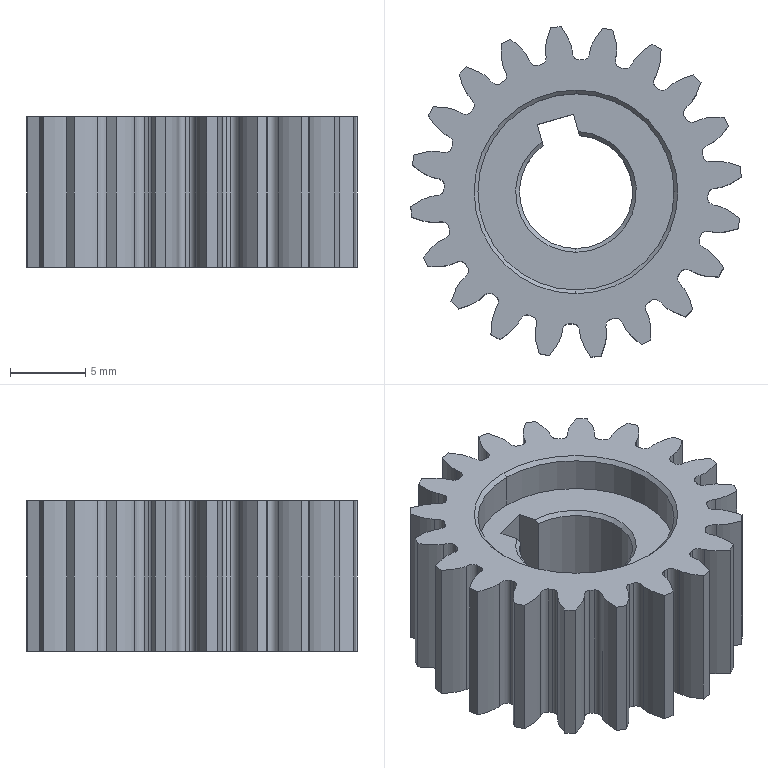Part | STEP file | GEAR_1_BODY-4 | 1 solid | 135 faces | box 21.911 x 21.911 x 10 mm | volume 2397 mm3 | spline 100 | cylinder 24 | plane 6 | cone 5 | commonest cylinder face diameters 17.5 x20 7.5 x2 13 x2